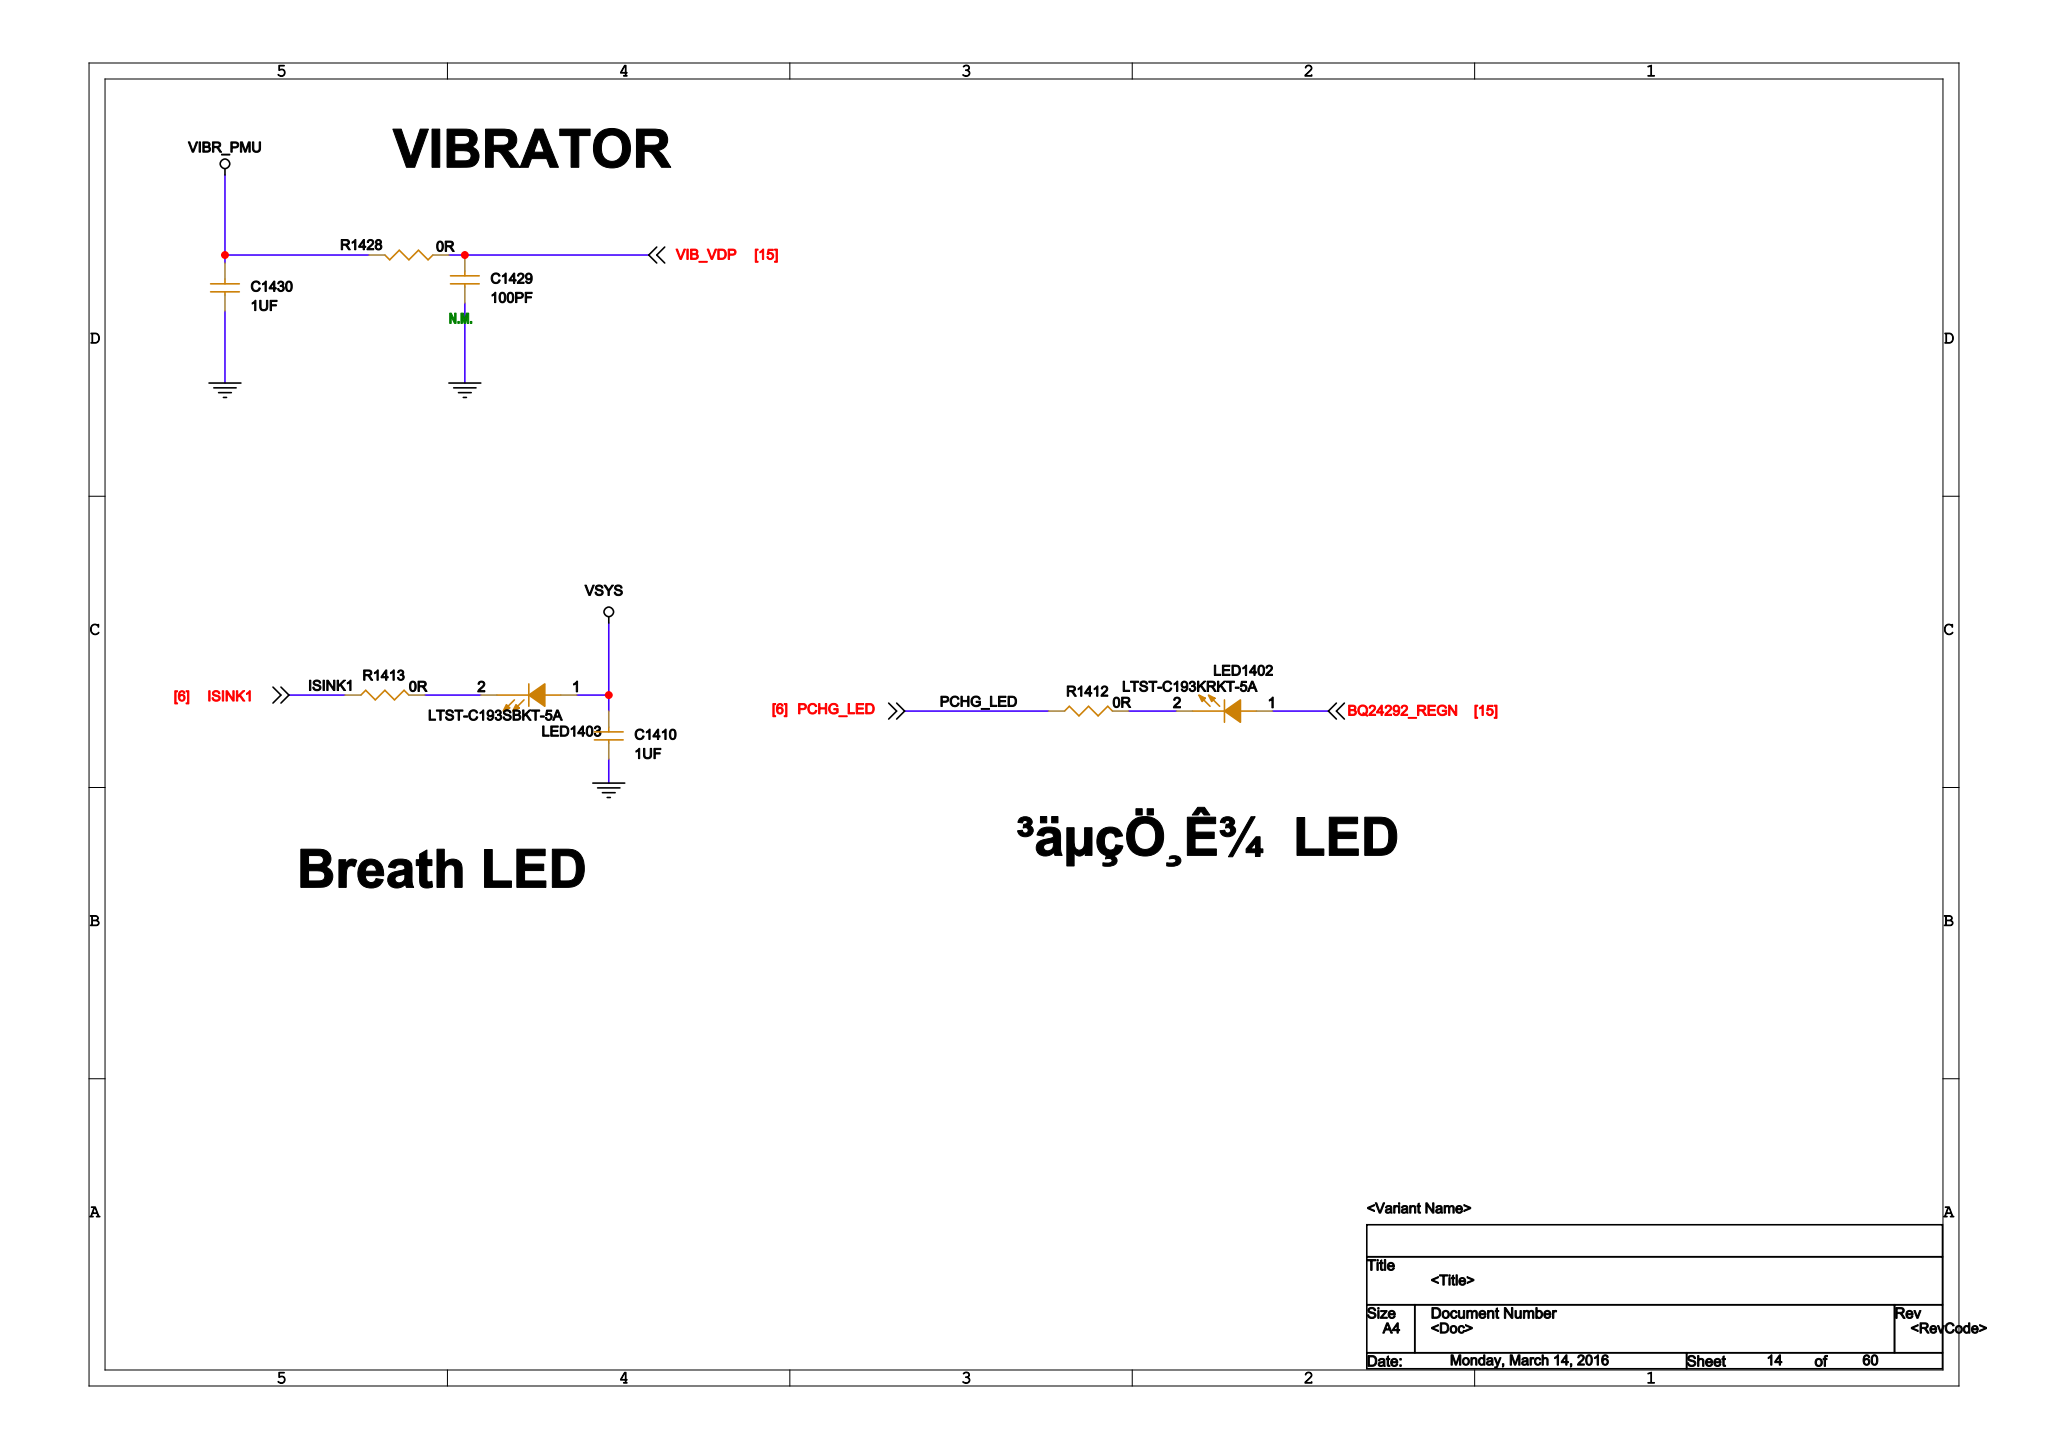Circuit board | Cadence Allegro | 1088 parts | 793 nets | one sheet of the schematic
Parts on this sheet (reference | value | footprint):
C1410 | 1UF | C0201
C1429
C1430 | 1UF | C0201
LED1402 | LTST-C193KRKT-5A | LED2_0P8X1P6X0P55_LITE-ON
LED1403 | LTST-C193SBKT-5A | LED2_0P8X1P6X0P55_LITE-ON
R1412 | 0R | R0201
R1413 | 0R | R0201
R1428 | 0R | R0201
Nets of these parts (net: part-pin ...):
GND: C1410-1 C1429-1 C1430-1
VSYS: C1410-2 LED1403-1
VIBR_PMU: C1430-2 R1428-2
BQ24292_REGN: LED1402-1
VIB_VDP: C1429-2 R1428-1
N33703376: LED1402-2 R1412-2
N33703378: LED1403-2 R1413-2
ISINK1: R1413-1
PCHG_LED: R1412-1